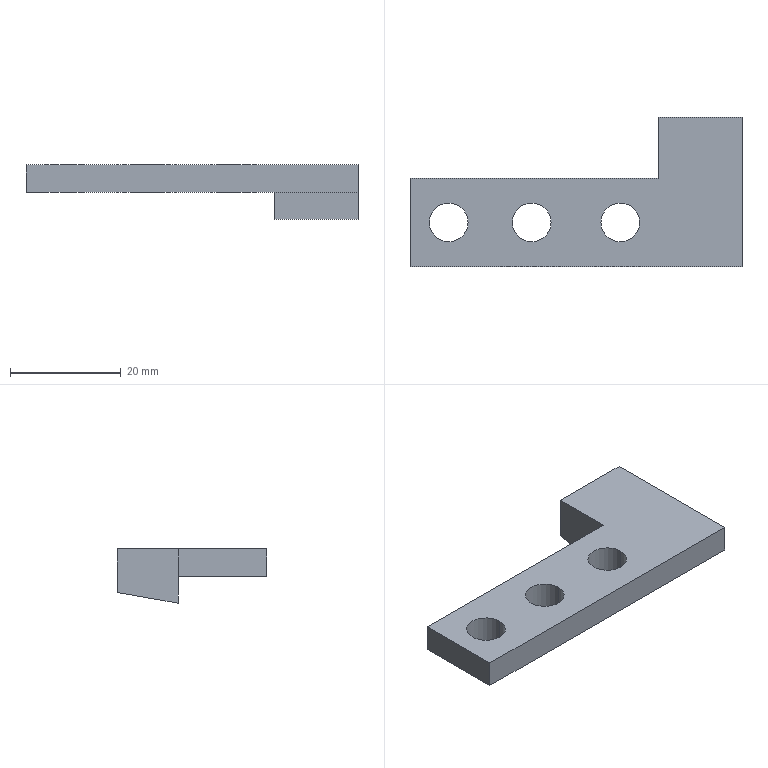Part | SolidWorks | features ICE 2, Extrusion 1 | 1 solid | 16 faces | box 60 x 27 x 9.83 mm | volume 5685 mm3 | plane 10 | cylinder 6 | commonest cylinder face diameters 7 x6
STEP:
#1=CARTESIAN_POINT('',(3.5,8.,-5.));
#2=VERTEX_POINT('',#1);
#3=CARTESIAN_POINT('',(10.5,8.,-5.));
#4=VERTEX_POINT('',#3);
#5=CARTESIAN_POINT('',(7.,8.,-5.));
#6=DIRECTION('',(0.,0.,1.));
#7=DIRECTION('',(0.,-1.,0.));
#8=AXIS2_PLACEMENT_3D('',#5,#6,#7);
#9=CIRCLE('',#8,3.5);
#10=EDGE_CURVE('',#2,#4,#9,.T.);
#11=ORIENTED_EDGE('',*,*,#10,.F.);
#12=CARTESIAN_POINT('',(3.5,8.,0.));
#13=VERTEX_POINT('',#12);
#14=CARTESIAN_POINT('',(3.5,8.,-60.));
#15=DIRECTION('',(0.,0.,1.));
#16=VECTOR('',#15,1000.);
#17=LINE('',#14,#16);
#18=EDGE_CURVE('',#2,#13,#17,.T.);
#19=ORIENTED_EDGE('',*,*,#18,.T.);
#20=CARTESIAN_POINT('',(10.5,8.,0.));
#21=VERTEX_POINT('',#20);
#22=CARTESIAN_POINT('',(7.,8.,0.));
#23=DIRECTION('',(0.,0.,1.));
#24=DIRECTION('',(1.,0.,0.));
#25=AXIS2_PLACEMENT_3D('',#22,#23,#24);
#26=CIRCLE('',#25,3.5);
#27=EDGE_CURVE('',#13,#21,#26,.T.);
#28=ORIENTED_EDGE('',*,*,#27,.T.);
#29=CARTESIAN_POINT('',(10.5,8.,-60.));
#30=DIRECTION('',(0.,0.,1.));
#31=VECTOR('',#30,1000.);
#32=LINE('',#29,#31);
#33=EDGE_CURVE('',#4,#21,#32,.T.);
#34=ORIENTED_EDGE('',*,*,#33,.F.);
#35=EDGE_LOOP('',(#11,#19,#28,#34));
#36=FACE_OUTER_BOUND('',#35,.T.);
#37=CARTESIAN_POINT('',(7.,8.,-60.));
#38=DIRECTION('',(0.,0.,1.));
#39=DIRECTION('',(1.,0.,0.));
#40=AXIS2_PLACEMENT_3D('',#37,#38,#39);
#41=CYLINDRICAL_SURFACE('',#40,3.5);
#42=ADVANCED_FACE('',(#36),#41,.F.);
#43=CARTESIAN_POINT('',(18.5,8.,-5.));
#44=VERTEX_POINT('',#43);
#45=CARTESIAN_POINT('',(25.5,8.,-5.));
#46=VERTEX_POINT('',#45);
#47=CARTESIAN_POINT('',(22.,8.,-5.));
#48=DIRECTION('',(0.,0.,1.));
#49=DIRECTION('',(0.,-1.,0.));
#50=AXIS2_PLACEMENT_3D('',#47,#48,#49);
#51=CIRCLE('',#50,3.5);
#52=EDGE_CURVE('',#44,#46,#51,.T.);
#53=ORIENTED_EDGE('',*,*,#52,.F.);
#54=CARTESIAN_POINT('',(18.5,8.,0.));
#55=VERTEX_POINT('',#54);
#56=CARTESIAN_POINT('',(18.5,8.,-60.));
#57=DIRECTION('',(0.,0.,1.));
#58=VECTOR('',#57,1000.);
#59=LINE('',#56,#58);
#60=EDGE_CURVE('',#44,#55,#59,.T.);
#61=ORIENTED_EDGE('',*,*,#60,.T.);
#62=CARTESIAN_POINT('',(25.5,8.,0.));
#63=VERTEX_POINT('',#62);
#64=CARTESIAN_POINT('',(22.,8.,0.));
#65=DIRECTION('',(0.,0.,1.));
#66=DIRECTION('',(1.,0.,0.));
#67=AXIS2_PLACEMENT_3D('',#64,#65,#66);
#68=CIRCLE('',#67,3.5);
#69=EDGE_CURVE('',#55,#63,#68,.T.);
#70=ORIENTED_EDGE('',*,*,#69,.T.);
#71=CARTESIAN_POINT('',(25.5,8.,-60.));
#72=DIRECTION('',(0.,0.,1.));
#73=VECTOR('',#72,1000.);
#74=LINE('',#71,#73);
#75=EDGE_CURVE('',#46,#63,#74,.T.);
#76=ORIENTED_EDGE('',*,*,#75,.F.);
#77=EDGE_LOOP('',(#53,#61,#70,#76));
#78=FACE_OUTER_BOUND('',#77,.T.);
#79=CARTESIAN_POINT('',(22.,8.,-60.));
#80=DIRECTION('',(0.,0.,1.));
#81=DIRECTION('',(1.,0.,0.));
#82=AXIS2_PLACEMENT_3D('',#79,#80,#81);
#83=CYLINDRICAL_SURFACE('',#82,3.5);
#84=ADVANCED_FACE('',(#78),#83,.F.);
#85=CARTESIAN_POINT('',(34.5,8.,-5.));
#86=VERTEX_POINT('',#85);
#87=CARTESIAN_POINT('',(41.5,8.,-5.));
#88=VERTEX_POINT('',#87);
#89=CARTESIAN_POINT('',(38.,8.,-5.));
#90=DIRECTION('',(0.,0.,1.));
#91=DIRECTION('',(0.,-1.,0.));
#92=AXIS2_PLACEMENT_3D('',#89,#90,#91);
#93=CIRCLE('',#92,3.5);
#94=EDGE_CURVE('',#86,#88,#93,.T.);
#95=ORIENTED_EDGE('',*,*,#94,.F.);
#96=CARTESIAN_POINT('',(34.5,8.,0.));
#97=VERTEX_POINT('',#96);
#98=CARTESIAN_POINT('',(34.5,8.,-60.));
#99=DIRECTION('',(0.,0.,1.));
#100=VECTOR('',#99,1000.);
#101=LINE('',#98,#100);
#102=EDGE_CURVE('',#86,#97,#101,.T.);
#103=ORIENTED_EDGE('',*,*,#102,.T.);
#104=CARTESIAN_POINT('',(41.5,8.,0.));
#105=VERTEX_POINT('',#104);
#106=CARTESIAN_POINT('',(38.,8.,0.));
#107=DIRECTION('',(0.,0.,1.));
#108=DIRECTION('',(1.,0.,0.));
#109=AXIS2_PLACEMENT_3D('',#106,#107,#108);
#110=CIRCLE('',#109,3.5);
#111=EDGE_CURVE('',#97,#105,#110,.T.);
#112=ORIENTED_EDGE('',*,*,#111,.T.);
#113=CARTESIAN_POINT('',(41.5,8.,-60.));
#114=DIRECTION('',(0.,0.,1.));
#115=VECTOR('',#114,1000.);
#116=LINE('',#113,#115);
#117=EDGE_CURVE('',#88,#105,#116,.T.);
#118=ORIENTED_EDGE('',*,*,#117,.F.);
#119=EDGE_LOOP('',(#95,#103,#112,#118));
#120=FACE_OUTER_BOUND('',#119,.T.);
#121=CARTESIAN_POINT('',(38.,8.,-60.));
#122=DIRECTION('',(0.,0.,1.));
#123=DIRECTION('',(1.,0.,0.));
#124=AXIS2_PLACEMENT_3D('',#121,#122,#123);
#125=CYLINDRICAL_SURFACE('',#124,3.5);
#126=ADVANCED_FACE('',(#120),#125,.F.);
#127=CARTESIAN_POINT('',(0.,0.,0.));
#128=VERTEX_POINT('',#127);
#129=CARTESIAN_POINT('',(0.,0.,-5.));
#130=VERTEX_POINT('',#129);
#131=CARTESIAN_POINT('',(0.,0.,-5.));
#132=DIRECTION('',(0.,0.,-1.));
#133=VECTOR('',#132,1000.);
#134=LINE('',#131,#133);
#135=EDGE_CURVE('',#128,#130,#134,.T.);
#136=ORIENTED_EDGE('',*,*,#135,.T.);
#137=CARTESIAN_POINT('',(60.,0.,-5.));
#138=VERTEX_POINT('',#137);
#139=CARTESIAN_POINT('',(60.,0.,-5.));
#140=DIRECTION('',(-1.,0.,0.));
#141=VECTOR('',#140,1000.);
#142=LINE('',#139,#141);
#143=EDGE_CURVE('',#138,#130,#142,.T.);
#144=ORIENTED_EDGE('',*,*,#143,.F.);
#145=CARTESIAN_POINT('',(60.,0.,0.));
#146=VERTEX_POINT('',#145);
#147=CARTESIAN_POINT('',(60.,0.,-5.));
#148=DIRECTION('',(0.,0.,-1.));
#149=VECTOR('',#148,1000.);
#150=LINE('',#147,#149);
#151=EDGE_CURVE('',#146,#138,#150,.T.);
#152=ORIENTED_EDGE('',*,*,#151,.F.);
#153=CARTESIAN_POINT('',(60.,0.,0.));
#154=DIRECTION('',(-1.,0.,0.));
#155=VECTOR('',#154,1000.);
#156=LINE('',#153,#155);
#157=EDGE_CURVE('',#146,#128,#156,.T.);
#158=ORIENTED_EDGE('',*,*,#157,.T.);
#159=EDGE_LOOP('',(#136,#144,#152,#158));
#160=FACE_OUTER_BOUND('',#159,.T.);
#161=CARTESIAN_POINT('',(60.,0.,-5.));
#162=DIRECTION('',(0.,1.,0.));
#163=DIRECTION('',(0.,0.,1.));
#164=AXIS2_PLACEMENT_3D('',#161,#162,#163);
#165=PLANE('',#164);
#166=ADVANCED_FACE('',(#160),#165,.F.);
#167=CARTESIAN_POINT('',(7.,8.,-5.));
#168=DIRECTION('',(0.,0.,1.));
#169=DIRECTION('',(0.,-1.,0.));
#170=AXIS2_PLACEMENT_3D('',#167,#168,#169);
#171=CIRCLE('',#170,3.5);
#172=EDGE_CURVE('',#4,#2,#171,.T.);
#173=ORIENTED_EDGE('',*,*,#172,.T.);
#174=ORIENTED_EDGE('',*,*,#10,.T.);
#175=EDGE_LOOP('',(#173,#174));
#176=FACE_BOUND('',#175,.T.);
#177=CARTESIAN_POINT('',(22.,8.,-5.));
#178=DIRECTION('',(0.,0.,1.));
#179=DIRECTION('',(0.,-1.,0.));
#180=AXIS2_PLACEMENT_3D('',#177,#178,#179);
#181=CIRCLE('',#180,3.5);
#182=EDGE_CURVE('',#46,#44,#181,.T.);
#183=ORIENTED_EDGE('',*,*,#182,.T.);
#184=ORIENTED_EDGE('',*,*,#52,.T.);
#185=EDGE_LOOP('',(#183,#184));
#186=FACE_BOUND('',#185,.T.);
#187=CARTESIAN_POINT('',(38.,8.,-5.));
#188=DIRECTION('',(0.,0.,1.));
#189=DIRECTION('',(0.,-1.,0.));
#190=AXIS2_PLACEMENT_3D('',#187,#188,#189);
#191=CIRCLE('',#190,3.5);
#192=EDGE_CURVE('',#88,#86,#191,.T.);
#193=ORIENTED_EDGE('',*,*,#192,.T.);
#194=ORIENTED_EDGE('',*,*,#94,.T.);
#195=EDGE_LOOP('',(#193,#194));
#196=FACE_BOUND('',#195,.T.);
#197=CARTESIAN_POINT('',(0.,16.,-5.));
#198=VERTEX_POINT('',#197);
#199=CARTESIAN_POINT('',(0.,16.,-5.));
#200=DIRECTION('',(0.,1.,0.));
#201=VECTOR('',#200,1000.);
#202=LINE('',#199,#201);
#203=EDGE_CURVE('',#130,#198,#202,.T.);
#204=ORIENTED_EDGE('',*,*,#203,.T.);
#205=CARTESIAN_POINT('',(45.,16.,-5.));
#206=VERTEX_POINT('',#205);
#207=CARTESIAN_POINT('',(60.,16.,-5.));
#208=DIRECTION('',(1.,0.,0.));
#209=VECTOR('',#208,1000.);
#210=LINE('',#207,#209);
#211=EDGE_CURVE('',#198,#206,#210,.T.);
#212=ORIENTED_EDGE('',*,*,#211,.T.);
#213=CARTESIAN_POINT('',(60.,16.,-5.));
#214=VERTEX_POINT('',#213);
#215=CARTESIAN_POINT('',(60.,16.,-5.));
#216=DIRECTION('',(-1.,0.,0.));
#217=VECTOR('',#216,1000.);
#218=LINE('',#215,#217);
#219=EDGE_CURVE('',#214,#206,#218,.T.);
#220=ORIENTED_EDGE('',*,*,#219,.F.);
#221=CARTESIAN_POINT('',(60.,16.,-5.));
#222=DIRECTION('',(0.,1.,0.));
#223=VECTOR('',#222,1000.);
#224=LINE('',#221,#223);
#225=EDGE_CURVE('',#138,#214,#224,.T.);
#226=ORIENTED_EDGE('',*,*,#225,.F.);
#227=ORIENTED_EDGE('',*,*,#143,.T.);
#228=EDGE_LOOP('',(#204,#212,#220,#226,#227));
#229=FACE_OUTER_BOUND('',#228,.T.);
#230=CARTESIAN_POINT('',(60.,16.,-5.));
#231=DIRECTION('',(0.,0.,1.));
#232=DIRECTION('',(0.,-1.,0.));
#233=AXIS2_PLACEMENT_3D('',#230,#231,#232);
#234=PLANE('',#233);
#235=ADVANCED_FACE('',(#176,#186,#196,#229),#234,.F.);
#236=ORIENTED_EDGE('',*,*,#219,.T.);
#237=CARTESIAN_POINT('',(45.,16.,-9.83));
#238=VERTEX_POINT('',#237);
#239=CARTESIAN_POINT('',(45.,16.,-60.));
#240=DIRECTION('',(0.,0.,1.));
#241=VECTOR('',#240,1000.);
#242=LINE('',#239,#241);
#243=EDGE_CURVE('',#238,#206,#242,.T.);
#244=ORIENTED_EDGE('',*,*,#243,.F.);
#245=CARTESIAN_POINT('',(60.,16.,-9.83));
#246=VERTEX_POINT('',#245);
#247=CARTESIAN_POINT('',(60.,16.,-9.83));
#248=DIRECTION('',(-1.,0.,0.));
#249=VECTOR('',#248,1000.);
#250=LINE('',#247,#249);
#251=EDGE_CURVE('',#246,#238,#250,.T.);
#252=ORIENTED_EDGE('',*,*,#251,.F.);
#253=CARTESIAN_POINT('',(60.,16.,-9.83));
#254=DIRECTION('',(0.,0.,-1.));
#255=VECTOR('',#254,1000.);
#256=LINE('',#253,#255);
#257=EDGE_CURVE('',#214,#246,#256,.T.);
#258=ORIENTED_EDGE('',*,*,#257,.F.);
#259=EDGE_LOOP('',(#236,#244,#252,#258));
#260=FACE_OUTER_BOUND('',#259,.T.);
#261=CARTESIAN_POINT('',(60.,16.,-9.83));
#262=DIRECTION('',(0.,1.,0.));
#263=DIRECTION('',(0.,0.,1.));
#264=AXIS2_PLACEMENT_3D('',#261,#262,#263);
#265=PLANE('',#264);
#266=ADVANCED_FACE('',(#260),#265,.F.);
#267=ORIENTED_EDGE('',*,*,#251,.T.);
#268=CARTESIAN_POINT('',(45.,27.,-7.89));
#269=VERTEX_POINT('',#268);
#270=CARTESIAN_POINT('',(45.,27.,-7.89));
#271=DIRECTION('',(0.,0.9848,0.1736));
#272=VECTOR('',#271,1000.);
#273=LINE('',#270,#272);
#274=EDGE_CURVE('',#238,#269,#273,.T.);
#275=ORIENTED_EDGE('',*,*,#274,.T.);
#276=CARTESIAN_POINT('',(60.,27.,-7.89));
#277=VERTEX_POINT('',#276);
#278=CARTESIAN_POINT('',(60.,27.,-7.89));
#279=DIRECTION('',(-1.,0.,0.));
#280=VECTOR('',#279,1000.);
#281=LINE('',#278,#280);
#282=EDGE_CURVE('',#277,#269,#281,.T.);
#283=ORIENTED_EDGE('',*,*,#282,.F.);
#284=CARTESIAN_POINT('',(60.,27.,-7.89));
#285=DIRECTION('',(0.,0.9848,0.1736));
#286=VECTOR('',#285,1000.);
#287=LINE('',#284,#286);
#288=EDGE_CURVE('',#246,#277,#287,.T.);
#289=ORIENTED_EDGE('',*,*,#288,.F.);
#290=EDGE_LOOP('',(#267,#275,#283,#289));
#291=FACE_OUTER_BOUND('',#290,.T.);
#292=CARTESIAN_POINT('',(60.,27.,-7.89));
#293=DIRECTION('',(0.,-0.1736,0.9848));
#294=DIRECTION('',(0.,-0.9848,-0.1736));
#295=AXIS2_PLACEMENT_3D('',#292,#293,#294);
#296=PLANE('',#295);
#297=ADVANCED_FACE('',(#291),#296,.F.);
#298=ORIENTED_EDGE('',*,*,#282,.T.);
#299=CARTESIAN_POINT('',(45.,27.,0.));
#300=VERTEX_POINT('',#299);
#301=CARTESIAN_POINT('',(45.,27.,-60.));
#302=DIRECTION('',(0.,0.,1.));
#303=VECTOR('',#302,1000.);
#304=LINE('',#301,#303);
#305=EDGE_CURVE('',#269,#300,#304,.T.);
#306=ORIENTED_EDGE('',*,*,#305,.T.);
#307=CARTESIAN_POINT('',(60.,27.,0.));
#308=VERTEX_POINT('',#307);
#309=CARTESIAN_POINT('',(60.,27.,0.));
#310=DIRECTION('',(-1.,0.,0.));
#311=VECTOR('',#310,1000.);
#312=LINE('',#309,#311);
#313=EDGE_CURVE('',#308,#300,#312,.T.);
#314=ORIENTED_EDGE('',*,*,#313,.F.);
#315=CARTESIAN_POINT('',(60.,27.,0.));
#316=DIRECTION('',(0.,0.,1.));
#317=VECTOR('',#316,1000.);
#318=LINE('',#315,#317);
#319=EDGE_CURVE('',#277,#308,#318,.T.);
#320=ORIENTED_EDGE('',*,*,#319,.F.);
#321=EDGE_LOOP('',(#298,#306,#314,#320));
#322=FACE_OUTER_BOUND('',#321,.T.);
#323=CARTESIAN_POINT('',(60.,27.,0.));
#324=DIRECTION('',(0.,-1.,0.));
#325=DIRECTION('',(0.,0.,-1.));
#326=AXIS2_PLACEMENT_3D('',#323,#324,#325);
#327=PLANE('',#326);
#328=ADVANCED_FACE('',(#322),#327,.F.);
#329=CARTESIAN_POINT('',(7.,8.,0.));
#330=DIRECTION('',(0.,0.,1.));
#331=DIRECTION('',(1.,0.,0.));
#332=AXIS2_PLACEMENT_3D('',#329,#330,#331);
#333=CIRCLE('',#332,3.5);
#334=EDGE_CURVE('',#21,#13,#333,.T.);
#335=ORIENTED_EDGE('',*,*,#334,.F.);
#336=ORIENTED_EDGE('',*,*,#27,.F.);
#337=EDGE_LOOP('',(#335,#336));
#338=FACE_BOUND('',#337,.T.);
#339=CARTESIAN_POINT('',(22.,8.,0.));
#340=DIRECTION('',(0.,0.,1.));
#341=DIRECTION('',(1.,0.,0.));
#342=AXIS2_PLACEMENT_3D('',#339,#340,#341);
#343=CIRCLE('',#342,3.5);
#344=EDGE_CURVE('',#63,#55,#343,.T.);
#345=ORIENTED_EDGE('',*,*,#344,.F.);
#346=ORIENTED_EDGE('',*,*,#69,.F.);
#347=EDGE_LOOP('',(#345,#346));
#348=FACE_BOUND('',#347,.T.);
#349=CARTESIAN_POINT('',(38.,8.,0.));
#350=DIRECTION('',(0.,0.,1.));
#351=DIRECTION('',(1.,0.,0.));
#352=AXIS2_PLACEMENT_3D('',#349,#350,#351);
#353=CIRCLE('',#352,3.5);
#354=EDGE_CURVE('',#105,#97,#353,.T.);
#355=ORIENTED_EDGE('',*,*,#354,.F.);
#356=ORIENTED_EDGE('',*,*,#111,.F.);
#357=EDGE_LOOP('',(#355,#356));
#358=FACE_BOUND('',#357,.T.);
#359=ORIENTED_EDGE('',*,*,#313,.T.);
#360=CARTESIAN_POINT('',(45.,16.,0.));
#361=VERTEX_POINT('',#360);
#362=CARTESIAN_POINT('',(45.,27.,0.));
#363=DIRECTION('',(0.,1.,0.));
#364=VECTOR('',#363,1000.);
#365=LINE('',#362,#364);
#366=EDGE_CURVE('',#361,#300,#365,.T.);
#367=ORIENTED_EDGE('',*,*,#366,.F.);
#368=CARTESIAN_POINT('',(0.,16.,0.));
#369=VERTEX_POINT('',#368);
#370=CARTESIAN_POINT('',(0.,16.,0.));
#371=DIRECTION('',(1.,0.,0.));
#372=VECTOR('',#371,1000.);
#373=LINE('',#370,#372);
#374=EDGE_CURVE('',#369,#361,#373,.T.);
#375=ORIENTED_EDGE('',*,*,#374,.F.);
#376=CARTESIAN_POINT('',(0.,0.,0.));
#377=DIRECTION('',(0.,-1.,0.));
#378=VECTOR('',#377,1000.);
#379=LINE('',#376,#378);
#380=EDGE_CURVE('',#369,#128,#379,.T.);
#381=ORIENTED_EDGE('',*,*,#380,.T.);
#382=ORIENTED_EDGE('',*,*,#157,.F.);
#383=CARTESIAN_POINT('',(60.,0.,0.));
#384=DIRECTION('',(0.,-1.,0.));
#385=VECTOR('',#384,1000.);
#386=LINE('',#383,#385);
#387=EDGE_CURVE('',#308,#146,#386,.T.);
#388=ORIENTED_EDGE('',*,*,#387,.F.);
#389=EDGE_LOOP('',(#359,#367,#375,#381,#382,#388));
#390=FACE_OUTER_BOUND('',#389,.T.);
#391=CARTESIAN_POINT('',(60.,0.,0.));
#392=DIRECTION('',(0.,0.,-1.));
#393=DIRECTION('',(-1.,0.,0.));
#394=AXIS2_PLACEMENT_3D('',#391,#392,#393);
#395=PLANE('',#394);
#396=ADVANCED_FACE('',(#338,#348,#358,#390),#395,.F.);
#397=ORIENTED_EDGE('',*,*,#151,.T.);
#398=ORIENTED_EDGE('',*,*,#225,.T.);
#399=ORIENTED_EDGE('',*,*,#257,.T.);
#400=ORIENTED_EDGE('',*,*,#288,.T.);
#401=ORIENTED_EDGE('',*,*,#319,.T.);
#402=ORIENTED_EDGE('',*,*,#387,.T.);
#403=EDGE_LOOP('',(#397,#398,#399,#400,#401,#402));
#404=FACE_OUTER_BOUND('',#403,.T.);
#405=CARTESIAN_POINT('',(60.,0.,0.));
#406=DIRECTION('',(-1.,0.,0.));
#407=DIRECTION('',(0.,0.,1.));
#408=AXIS2_PLACEMENT_3D('',#405,#406,#407);
#409=PLANE('',#408);
#410=ADVANCED_FACE('',(#404),#409,.F.);
#411=CARTESIAN_POINT('',(0.,16.,0.));
#412=DIRECTION('',(0.,0.,1.));
#413=VECTOR('',#412,1000.);
#414=LINE('',#411,#413);
#415=EDGE_CURVE('',#198,#369,#414,.T.);
#416=ORIENTED_EDGE('',*,*,#415,.F.);
#417=ORIENTED_EDGE('',*,*,#203,.F.);
#418=ORIENTED_EDGE('',*,*,#135,.F.);
#419=ORIENTED_EDGE('',*,*,#380,.F.);
#420=EDGE_LOOP('',(#416,#417,#418,#419));
#421=FACE_OUTER_BOUND('',#420,.T.);
#422=CARTESIAN_POINT('',(0.,0.,0.));
#423=DIRECTION('',(-1.,0.,0.));
#424=DIRECTION('',(0.,0.,1.));
#425=AXIS2_PLACEMENT_3D('',#422,#423,#424);
#426=PLANE('',#425);
#427=ADVANCED_FACE('',(#421),#426,.T.);
#428=ORIENTED_EDGE('',*,*,#243,.T.);
#429=CARTESIAN_POINT('',(45.,16.,-60.));
#430=DIRECTION('',(0.,0.,1.));
#431=VECTOR('',#430,1000.);
#432=LINE('',#429,#431);
#433=EDGE_CURVE('',#206,#361,#432,.T.);
#434=ORIENTED_EDGE('',*,*,#433,.T.);
#435=ORIENTED_EDGE('',*,*,#366,.T.);
#436=ORIENTED_EDGE('',*,*,#305,.F.);
#437=ORIENTED_EDGE('',*,*,#274,.F.);
#438=EDGE_LOOP('',(#428,#434,#435,#436,#437));
#439=FACE_OUTER_BOUND('',#438,.T.);
#440=CARTESIAN_POINT('',(45.,27.,-60.));
#441=DIRECTION('',(1.,0.,0.));
#442=DIRECTION('',(0.,0.,-1.));
#443=AXIS2_PLACEMENT_3D('',#440,#441,#442);
#444=PLANE('',#443);
#445=ADVANCED_FACE('',(#439),#444,.F.);
#446=ORIENTED_EDGE('',*,*,#415,.T.);
#447=ORIENTED_EDGE('',*,*,#374,.T.);
#448=ORIENTED_EDGE('',*,*,#433,.F.);
#449=ORIENTED_EDGE('',*,*,#211,.F.);
#450=EDGE_LOOP('',(#446,#447,#448,#449));
#451=FACE_OUTER_BOUND('',#450,.T.);
#452=CARTESIAN_POINT('',(0.,16.,-60.));
#453=DIRECTION('',(0.,-1.,0.));
#454=DIRECTION('',(0.,0.,-1.));
#455=AXIS2_PLACEMENT_3D('',#452,#453,#454);
#456=PLANE('',#455);
#457=ADVANCED_FACE('',(#451),#456,.F.);
#458=ORIENTED_EDGE('',*,*,#102,.F.);
#459=ORIENTED_EDGE('',*,*,#192,.F.);
#460=ORIENTED_EDGE('',*,*,#117,.T.);
#461=ORIENTED_EDGE('',*,*,#354,.T.);
#462=EDGE_LOOP('',(#458,#459,#460,#461));
#463=FACE_OUTER_BOUND('',#462,.T.);
#464=CARTESIAN_POINT('',(38.,8.,-60.));
#465=DIRECTION('',(0.,0.,1.));
#466=DIRECTION('',(1.,0.,0.));
#467=AXIS2_PLACEMENT_3D('',#464,#465,#466);
#468=CYLINDRICAL_SURFACE('',#467,3.5);
#469=ADVANCED_FACE('',(#463),#468,.F.);
#470=ORIENTED_EDGE('',*,*,#60,.F.);
#471=ORIENTED_EDGE('',*,*,#182,.F.);
#472=ORIENTED_EDGE('',*,*,#75,.T.);
#473=ORIENTED_EDGE('',*,*,#344,.T.);
#474=EDGE_LOOP('',(#470,#471,#472,#473));
#475=FACE_OUTER_BOUND('',#474,.T.);
#476=CARTESIAN_POINT('',(22.,8.,-60.));
#477=DIRECTION('',(0.,0.,1.));
#478=DIRECTION('',(1.,0.,0.));
#479=AXIS2_PLACEMENT_3D('',#476,#477,#478);
#480=CYLINDRICAL_SURFACE('',#479,3.5);
#481=ADVANCED_FACE('',(#475),#480,.F.);
#482=ORIENTED_EDGE('',*,*,#18,.F.);
#483=ORIENTED_EDGE('',*,*,#172,.F.);
#484=ORIENTED_EDGE('',*,*,#33,.T.);
#485=ORIENTED_EDGE('',*,*,#334,.T.);
#486=EDGE_LOOP('',(#482,#483,#484,#485));
#487=FACE_OUTER_BOUND('',#486,.T.);
#488=CARTESIAN_POINT('',(7.,8.,-60.));
#489=DIRECTION('',(0.,0.,1.));
#490=DIRECTION('',(1.,0.,0.));
#491=AXIS2_PLACEMENT_3D('',#488,#489,#490);
#492=CYLINDRICAL_SURFACE('',#491,3.5);
#493=ADVANCED_FACE('',(#487),#492,.F.);
#494=CLOSED_SHELL('',(#42,#84,#126,#166,#235,#266,#297,#328,#396,#410,#427,#445,#457,#469,#481,#493));
#495=MANIFOLD_SOLID_BREP('',#494);
#496=CARTESIAN_POINT('',(0.,0.,0.));
#497=DIRECTION('',(0.,0.,1.));
#498=DIRECTION('',(1.,0.,0.));
#499=AXIS2_PLACEMENT_3D('',#496,#497,#498);
#500=(LENGTH_UNIT()NAMED_UNIT(*)SI_UNIT(.MILLI.,.METRE.));
#501=UNCERTAINTY_MEASURE_WITH_UNIT(LENGTH_MEASURE(0.00001),#500,'','');
#502=(NAMED_UNIT(*)PLANE_ANGLE_UNIT()SI_UNIT($,.RADIAN.));
#503=(NAMED_UNIT(*)SI_UNIT($,.STERADIAN.)SOLID_ANGLE_UNIT());
#504=(GEOMETRIC_REPRESENTATION_CONTEXT(3)GLOBAL_UNCERTAINTY_ASSIGNED_CONTEXT((#501))GLOBAL_UNIT_ASSIGNED_CONTEXT((#500,#502,#503))REPRESENTATION_CONTEXT('',''));
#505=ADVANCED_BREP_SHAPE_REPRESENTATION('',(#495,#499),#504);